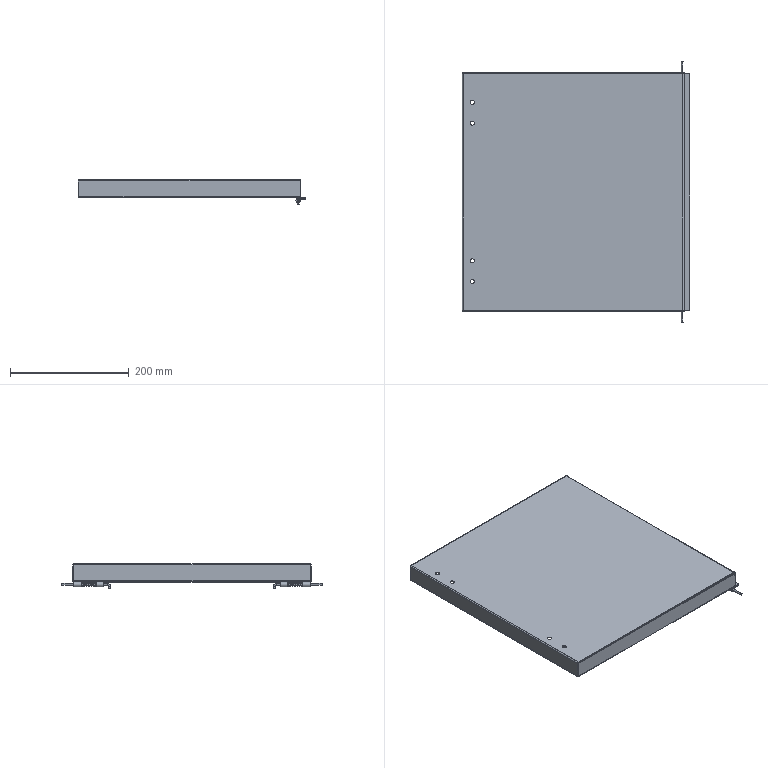Part | 5 solids | 145 faces | box 383.8 x 438.127 x 41 mm | volume 255227 mm3 | plane 76 | cylinder 51 | spline 14 | torus 4 | commonest cylinder face diameters 7 x11 1.473 x8 3 x8 3.6 x8 3.873 x8 7.6 x8